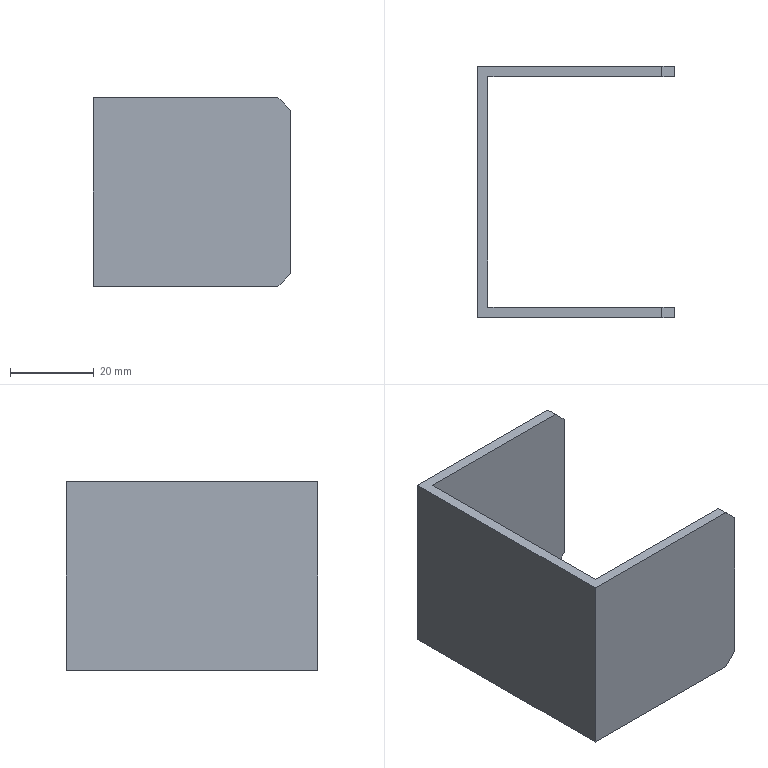Part | SolidWorks | features BaseBody 1 | 1 solid | 14 faces | box 47 x 60 x 45 mm | volume 16717 mm3 | plane 14
STEP:
#1=CARTESIAN_POINT('',(896.946,-3035.973,2067.471));
#2=VERTEX_POINT('',#1);
#3=CARTESIAN_POINT('',(896.946,-3095.973,2067.471));
#4=VERTEX_POINT('',#3);
#5=CARTESIAN_POINT('',(896.946,-3035.973,2067.471));
#6=DIRECTION('',(0.,-1.,0.));
#7=VECTOR('',#6,1000.);
#8=LINE('',#5,#7);
#9=EDGE_CURVE('',#2,#4,#8,.T.);
#10=ORIENTED_EDGE('',*,*,#9,.T.);
#11=CARTESIAN_POINT('',(896.946,-3095.973,2112.471));
#12=VERTEX_POINT('',#11);
#13=CARTESIAN_POINT('',(896.946,-3095.973,2067.471));
#14=DIRECTION('',(0.,0.,1.));
#15=VECTOR('',#14,1000.);
#16=LINE('',#13,#15);
#17=EDGE_CURVE('',#4,#12,#16,.T.);
#18=ORIENTED_EDGE('',*,*,#17,.T.);
#19=CARTESIAN_POINT('',(896.946,-3035.973,2112.471));
#20=VERTEX_POINT('',#19);
#21=CARTESIAN_POINT('',(896.946,-3035.973,2112.471));
#22=DIRECTION('',(0.,1.,0.));
#23=VECTOR('',#22,1000.);
#24=LINE('',#21,#23);
#25=EDGE_CURVE('',#12,#20,#24,.T.);
#26=ORIENTED_EDGE('',*,*,#25,.T.);
#27=CARTESIAN_POINT('',(896.946,-3035.973,2067.471));
#28=DIRECTION('',(0.,0.,-1.));
#29=VECTOR('',#28,1000.);
#30=LINE('',#27,#29);
#31=EDGE_CURVE('',#20,#2,#30,.T.);
#32=ORIENTED_EDGE('',*,*,#31,.T.);
#33=EDGE_LOOP('',(#10,#18,#26,#32));
#34=FACE_OUTER_BOUND('',#33,.T.);
#35=CARTESIAN_POINT('',(896.946,-3035.973,2067.471));
#36=DIRECTION('',(-1.,0.,0.));
#37=DIRECTION('',(0.,0.,1.));
#38=AXIS2_PLACEMENT_3D('',#35,#36,#37);
#39=PLANE('',#38);
#40=ADVANCED_FACE('',(#34),#39,.T.);
#41=CARTESIAN_POINT('',(940.946,-3095.973,2067.471));
#42=VERTEX_POINT('',#41);
#43=CARTESIAN_POINT('',(943.946,-3095.973,2070.471));
#44=VERTEX_POINT('',#43);
#45=CARTESIAN_POINT('',(940.946,-3095.973,2067.471));
#46=DIRECTION('',(0.7071,0.,0.7071));
#47=VECTOR('',#46,1000.);
#48=LINE('',#45,#47);
#49=EDGE_CURVE('',#42,#44,#48,.T.);
#50=ORIENTED_EDGE('',*,*,#49,.T.);
#51=CARTESIAN_POINT('',(943.946,-3095.973,2109.471));
#52=VERTEX_POINT('',#51);
#53=CARTESIAN_POINT('',(943.946,-3095.973,2067.471));
#54=DIRECTION('',(0.,0.,1.));
#55=VECTOR('',#54,1000.);
#56=LINE('',#53,#55);
#57=EDGE_CURVE('',#44,#52,#56,.T.);
#58=ORIENTED_EDGE('',*,*,#57,.T.);
#59=CARTESIAN_POINT('',(940.946,-3095.973,2112.471));
#60=VERTEX_POINT('',#59);
#61=CARTESIAN_POINT('',(943.946,-3095.973,2109.471));
#62=DIRECTION('',(-0.7071,0.,0.7071));
#63=VECTOR('',#62,1000.);
#64=LINE('',#61,#63);
#65=EDGE_CURVE('',#52,#60,#64,.T.);
#66=ORIENTED_EDGE('',*,*,#65,.T.);
#67=CARTESIAN_POINT('',(896.946,-3095.973,2112.471));
#68=DIRECTION('',(-1.,0.,0.));
#69=VECTOR('',#68,1000.);
#70=LINE('',#67,#69);
#71=EDGE_CURVE('',#60,#12,#70,.T.);
#72=ORIENTED_EDGE('',*,*,#71,.T.);
#73=ORIENTED_EDGE('',*,*,#17,.F.);
#74=CARTESIAN_POINT('',(896.946,-3095.973,2067.471));
#75=DIRECTION('',(1.,0.,0.));
#76=VECTOR('',#75,1000.);
#77=LINE('',#74,#76);
#78=EDGE_CURVE('',#4,#42,#77,.T.);
#79=ORIENTED_EDGE('',*,*,#78,.T.);
#80=EDGE_LOOP('',(#50,#58,#66,#72,#73,#79));
#81=FACE_OUTER_BOUND('',#80,.T.);
#82=CARTESIAN_POINT('',(896.946,-3095.973,2067.471));
#83=DIRECTION('',(0.,-1.,0.));
#84=DIRECTION('',(0.,0.,-1.));
#85=AXIS2_PLACEMENT_3D('',#82,#83,#84);
#86=PLANE('',#85);
#87=ADVANCED_FACE('',(#81),#86,.T.);
#88=CARTESIAN_POINT('',(899.446,-3038.473,2067.471));
#89=VERTEX_POINT('',#88);
#90=CARTESIAN_POINT('',(940.946,-3038.473,2067.471));
#91=VERTEX_POINT('',#90);
#92=CARTESIAN_POINT('',(912.735,-3038.473,2067.471));
#93=DIRECTION('',(1.,0.,0.));
#94=VECTOR('',#93,1000.);
#95=LINE('',#92,#94);
#96=EDGE_CURVE('',#89,#91,#95,.T.);
#97=ORIENTED_EDGE('',*,*,#96,.F.);
#98=CARTESIAN_POINT('',(899.446,-3093.473,2067.471));
#99=VERTEX_POINT('',#98);
#100=CARTESIAN_POINT('',(899.446,-3065.973,2067.471));
#101=DIRECTION('',(0.,1.,0.));
#102=VECTOR('',#101,1000.);
#103=LINE('',#100,#102);
#104=EDGE_CURVE('',#99,#89,#103,.T.);
#105=ORIENTED_EDGE('',*,*,#104,.F.);
#106=CARTESIAN_POINT('',(940.946,-3093.473,2067.471));
#107=VERTEX_POINT('',#106);
#108=CARTESIAN_POINT('',(912.735,-3093.473,2067.471));
#109=DIRECTION('',(-1.,0.,0.));
#110=VECTOR('',#109,1000.);
#111=LINE('',#108,#110);
#112=EDGE_CURVE('',#107,#99,#111,.T.);
#113=ORIENTED_EDGE('',*,*,#112,.F.);
#114=CARTESIAN_POINT('',(940.946,-3065.973,2067.471));
#115=DIRECTION('',(0.,1.,0.));
#116=VECTOR('',#115,1000.);
#117=LINE('',#114,#116);
#118=EDGE_CURVE('',#42,#107,#117,.T.);
#119=ORIENTED_EDGE('',*,*,#118,.F.);
#120=ORIENTED_EDGE('',*,*,#78,.F.);
#121=ORIENTED_EDGE('',*,*,#9,.F.);
#122=CARTESIAN_POINT('',(940.946,-3035.973,2067.471));
#123=VERTEX_POINT('',#122);
#124=CARTESIAN_POINT('',(912.735,-3035.973,2067.471));
#125=DIRECTION('',(-1.,0.,0.));
#126=VECTOR('',#125,1000.);
#127=LINE('',#124,#126);
#128=EDGE_CURVE('',#123,#2,#127,.T.);
#129=ORIENTED_EDGE('',*,*,#128,.F.);
#130=CARTESIAN_POINT('',(940.946,-3065.973,2067.471));
#131=DIRECTION('',(0.,1.,0.));
#132=VECTOR('',#131,1000.);
#133=LINE('',#130,#132);
#134=EDGE_CURVE('',#91,#123,#133,.T.);
#135=ORIENTED_EDGE('',*,*,#134,.F.);
#136=EDGE_LOOP('',(#97,#105,#113,#119,#120,#121,#129,#135));
#137=FACE_OUTER_BOUND('',#136,.T.);
#138=CARTESIAN_POINT('',(912.735,-3065.973,2067.471));
#139=DIRECTION('',(0.,0.,1.));
#140=DIRECTION('',(1.,0.,0.));
#141=AXIS2_PLACEMENT_3D('',#138,#139,#140);
#142=PLANE('',#141);
#143=ADVANCED_FACE('',(#137),#142,.F.);
#144=ORIENTED_EDGE('',*,*,#31,.F.);
#145=CARTESIAN_POINT('',(940.946,-3035.973,2112.471));
#146=VERTEX_POINT('',#145);
#147=CARTESIAN_POINT('',(943.946,-3035.973,2112.471));
#148=DIRECTION('',(1.,0.,0.));
#149=VECTOR('',#148,1000.);
#150=LINE('',#147,#149);
#151=EDGE_CURVE('',#20,#146,#150,.T.);
#152=ORIENTED_EDGE('',*,*,#151,.T.);
#153=CARTESIAN_POINT('',(943.946,-3035.973,2109.471));
#154=VERTEX_POINT('',#153);
#155=CARTESIAN_POINT('',(940.946,-3035.973,2112.471));
#156=DIRECTION('',(0.7071,0.,-0.7071));
#157=VECTOR('',#156,1000.);
#158=LINE('',#155,#157);
#159=EDGE_CURVE('',#146,#154,#158,.T.);
#160=ORIENTED_EDGE('',*,*,#159,.T.);
#161=CARTESIAN_POINT('',(943.946,-3035.973,2070.471));
#162=VERTEX_POINT('',#161);
#163=CARTESIAN_POINT('',(943.946,-3035.973,2067.471));
#164=DIRECTION('',(0.,0.,-1.));
#165=VECTOR('',#164,1000.);
#166=LINE('',#163,#165);
#167=EDGE_CURVE('',#154,#162,#166,.T.);
#168=ORIENTED_EDGE('',*,*,#167,.T.);
#169=CARTESIAN_POINT('',(943.946,-3035.973,2070.471));
#170=DIRECTION('',(-0.7071,0.,-0.7071));
#171=VECTOR('',#170,1000.);
#172=LINE('',#169,#171);
#173=EDGE_CURVE('',#162,#123,#172,.T.);
#174=ORIENTED_EDGE('',*,*,#173,.T.);
#175=ORIENTED_EDGE('',*,*,#128,.T.);
#176=EDGE_LOOP('',(#144,#152,#160,#168,#174,#175));
#177=FACE_OUTER_BOUND('',#176,.T.);
#178=CARTESIAN_POINT('',(943.946,-3035.973,2067.471));
#179=DIRECTION('',(0.,1.,0.));
#180=DIRECTION('',(0.,0.,1.));
#181=AXIS2_PLACEMENT_3D('',#178,#179,#180);
#182=PLANE('',#181);
#183=ADVANCED_FACE('',(#177),#182,.T.);
#184=CARTESIAN_POINT('',(899.446,-3093.473,2112.471));
#185=VERTEX_POINT('',#184);
#186=CARTESIAN_POINT('',(899.446,-3038.473,2112.471));
#187=VERTEX_POINT('',#186);
#188=CARTESIAN_POINT('',(899.446,-3065.973,2112.471));
#189=DIRECTION('',(0.,1.,0.));
#190=VECTOR('',#189,1000.);
#191=LINE('',#188,#190);
#192=EDGE_CURVE('',#185,#187,#191,.T.);
#193=ORIENTED_EDGE('',*,*,#192,.T.);
#194=CARTESIAN_POINT('',(940.946,-3038.473,2112.471));
#195=VERTEX_POINT('',#194);
#196=CARTESIAN_POINT('',(912.735,-3038.473,2112.471));
#197=DIRECTION('',(1.,0.,0.));
#198=VECTOR('',#197,1000.);
#199=LINE('',#196,#198);
#200=EDGE_CURVE('',#187,#195,#199,.T.);
#201=ORIENTED_EDGE('',*,*,#200,.T.);
#202=CARTESIAN_POINT('',(940.946,-3065.973,2112.471));
#203=DIRECTION('',(0.,1.,0.));
#204=VECTOR('',#203,1000.);
#205=LINE('',#202,#204);
#206=EDGE_CURVE('',#195,#146,#205,.T.);
#207=ORIENTED_EDGE('',*,*,#206,.T.);
#208=ORIENTED_EDGE('',*,*,#151,.F.);
#209=ORIENTED_EDGE('',*,*,#25,.F.);
#210=ORIENTED_EDGE('',*,*,#71,.F.);
#211=CARTESIAN_POINT('',(940.946,-3093.473,2112.471));
#212=VERTEX_POINT('',#211);
#213=CARTESIAN_POINT('',(940.946,-3065.973,2112.471));
#214=DIRECTION('',(0.,1.,0.));
#215=VECTOR('',#214,1000.);
#216=LINE('',#213,#215);
#217=EDGE_CURVE('',#60,#212,#216,.T.);
#218=ORIENTED_EDGE('',*,*,#217,.T.);
#219=CARTESIAN_POINT('',(912.735,-3093.473,2112.471));
#220=DIRECTION('',(-1.,0.,0.));
#221=VECTOR('',#220,1000.);
#222=LINE('',#219,#221);
#223=EDGE_CURVE('',#212,#185,#222,.T.);
#224=ORIENTED_EDGE('',*,*,#223,.T.);
#225=EDGE_LOOP('',(#193,#201,#207,#208,#209,#210,#218,#224));
#226=FACE_OUTER_BOUND('',#225,.T.);
#227=CARTESIAN_POINT('',(912.735,-3065.973,2112.471));
#228=DIRECTION('',(0.,0.,1.));
#229=DIRECTION('',(1.,0.,0.));
#230=AXIS2_PLACEMENT_3D('',#227,#228,#229);
#231=PLANE('',#230);
#232=ADVANCED_FACE('',(#226),#231,.T.);
#233=CARTESIAN_POINT('',(943.946,-3093.473,2070.471));
#234=VERTEX_POINT('',#233);
#235=CARTESIAN_POINT('',(943.946,-3095.973,2070.471));
#236=DIRECTION('',(0.,1.,0.));
#237=VECTOR('',#236,1000.);
#238=LINE('',#235,#237);
#239=EDGE_CURVE('',#44,#234,#238,.T.);
#240=ORIENTED_EDGE('',*,*,#239,.T.);
#241=CARTESIAN_POINT('',(943.946,-3093.473,2109.471));
#242=VERTEX_POINT('',#241);
#243=CARTESIAN_POINT('',(943.946,-3093.473,2067.471));
#244=DIRECTION('',(0.,0.,1.));
#245=VECTOR('',#244,1000.);
#246=LINE('',#243,#245);
#247=EDGE_CURVE('',#234,#242,#246,.T.);
#248=ORIENTED_EDGE('',*,*,#247,.T.);
#249=CARTESIAN_POINT('',(943.946,-3095.973,2109.471));
#250=DIRECTION('',(0.,-1.,0.));
#251=VECTOR('',#250,1000.);
#252=LINE('',#249,#251);
#253=EDGE_CURVE('',#242,#52,#252,.T.);
#254=ORIENTED_EDGE('',*,*,#253,.T.);
#255=ORIENTED_EDGE('',*,*,#57,.F.);
#256=EDGE_LOOP('',(#240,#248,#254,#255));
#257=FACE_OUTER_BOUND('',#256,.T.);
#258=CARTESIAN_POINT('',(943.946,-3095.973,2067.471));
#259=DIRECTION('',(1.,0.,0.));
#260=DIRECTION('',(0.,0.,-1.));
#261=AXIS2_PLACEMENT_3D('',#258,#259,#260);
#262=PLANE('',#261);
#263=ADVANCED_FACE('',(#257),#262,.T.);
#264=ORIENTED_EDGE('',*,*,#118,.T.);
#265=CARTESIAN_POINT('',(943.946,-3093.473,2070.471));
#266=DIRECTION('',(-0.7071,0.,-0.7071));
#267=VECTOR('',#266,1000.);
#268=LINE('',#265,#267);
#269=EDGE_CURVE('',#234,#107,#268,.T.);
#270=ORIENTED_EDGE('',*,*,#269,.F.);
#271=ORIENTED_EDGE('',*,*,#239,.F.);
#272=ORIENTED_EDGE('',*,*,#49,.F.);
#273=EDGE_LOOP('',(#264,#270,#271,#272));
#274=FACE_OUTER_BOUND('',#273,.T.);
#275=CARTESIAN_POINT('',(943.946,-2900.175,2070.471));
#276=DIRECTION('',(-0.7071,0.,0.7071));
#277=DIRECTION('',(0.7071,0.,0.7071));
#278=AXIS2_PLACEMENT_3D('',#275,#276,#277);
#279=PLANE('',#278);
#280=ADVANCED_FACE('',(#274),#279,.F.);
#281=ORIENTED_EDGE('',*,*,#253,.F.);
#282=CARTESIAN_POINT('',(943.946,-3093.473,2109.471));
#283=DIRECTION('',(0.7071,0.,-0.7071));
#284=VECTOR('',#283,1000.);
#285=LINE('',#282,#284);
#286=EDGE_CURVE('',#212,#242,#285,.T.);
#287=ORIENTED_EDGE('',*,*,#286,.F.);
#288=ORIENTED_EDGE('',*,*,#217,.F.);
#289=ORIENTED_EDGE('',*,*,#65,.F.);
#290=EDGE_LOOP('',(#281,#287,#288,#289));
#291=FACE_OUTER_BOUND('',#290,.T.);
#292=CARTESIAN_POINT('',(943.946,-2900.175,2109.471));
#293=DIRECTION('',(-0.7071,0.,-0.7071));
#294=DIRECTION('',(-0.7071,0.,0.7071));
#295=AXIS2_PLACEMENT_3D('',#292,#293,#294);
#296=PLANE('',#295);
#297=ADVANCED_FACE('',(#291),#296,.F.);
#298=CARTESIAN_POINT('',(943.946,-3038.473,2070.471));
#299=VERTEX_POINT('',#298);
#300=CARTESIAN_POINT('',(943.946,-2900.175,2070.471));
#301=DIRECTION('',(0.,1.,0.));
#302=VECTOR('',#301,1000.);
#303=LINE('',#300,#302);
#304=EDGE_CURVE('',#299,#162,#303,.T.);
#305=ORIENTED_EDGE('',*,*,#304,.F.);
#306=CARTESIAN_POINT('',(943.946,-3038.473,2070.471));
#307=DIRECTION('',(0.7071,0.,0.7071));
#308=VECTOR('',#307,1000.);
#309=LINE('',#306,#308);
#310=EDGE_CURVE('',#91,#299,#309,.T.);
#311=ORIENTED_EDGE('',*,*,#310,.F.);
#312=ORIENTED_EDGE('',*,*,#134,.T.);
#313=ORIENTED_EDGE('',*,*,#173,.F.);
#314=EDGE_LOOP('',(#305,#311,#312,#313));
#315=FACE_OUTER_BOUND('',#314,.T.);
#316=CARTESIAN_POINT('',(943.946,-2900.175,2070.471));
#317=DIRECTION('',(-0.7071,0.,0.7071));
#318=DIRECTION('',(0.7071,0.,0.7071));
#319=AXIS2_PLACEMENT_3D('',#316,#317,#318);
#320=PLANE('',#319);
#321=ADVANCED_FACE('',(#315),#320,.F.);
#322=ORIENTED_EDGE('',*,*,#310,.T.);
#323=CARTESIAN_POINT('',(943.946,-3038.473,2109.471));
#324=VERTEX_POINT('',#323);
#325=CARTESIAN_POINT('',(943.946,-3038.473,2067.471));
#326=DIRECTION('',(0.,0.,1.));
#327=VECTOR('',#326,1000.);
#328=LINE('',#325,#327);
#329=EDGE_CURVE('',#299,#324,#328,.T.);
#330=ORIENTED_EDGE('',*,*,#329,.T.);
#331=CARTESIAN_POINT('',(943.946,-3038.473,2109.471));
#332=DIRECTION('',(-0.7071,0.,0.7071));
#333=VECTOR('',#332,1000.);
#334=LINE('',#331,#333);
#335=EDGE_CURVE('',#324,#195,#334,.T.);
#336=ORIENTED_EDGE('',*,*,#335,.T.);
#337=ORIENTED_EDGE('',*,*,#200,.F.);
#338=CARTESIAN_POINT('',(899.446,-3038.473,2067.471));
#339=DIRECTION('',(0.,0.,-1.));
#340=VECTOR('',#339,1000.);
#341=LINE('',#338,#340);
#342=EDGE_CURVE('',#187,#89,#341,.T.);
#343=ORIENTED_EDGE('',*,*,#342,.T.);
#344=ORIENTED_EDGE('',*,*,#96,.T.);
#345=EDGE_LOOP('',(#322,#330,#336,#337,#343,#344));
#346=FACE_OUTER_BOUND('',#345,.T.);
#347=CARTESIAN_POINT('',(899.446,-3038.473,2067.471));
#348=DIRECTION('',(0.,-1.,0.));
#349=DIRECTION('',(0.,0.,-1.));
#350=AXIS2_PLACEMENT_3D('',#347,#348,#349);
#351=PLANE('',#350);
#352=ADVANCED_FACE('',(#346),#351,.T.);
#353=ORIENTED_EDGE('',*,*,#104,.T.);
#354=ORIENTED_EDGE('',*,*,#342,.F.);
#355=ORIENTED_EDGE('',*,*,#192,.F.);
#356=CARTESIAN_POINT('',(899.446,-3093.473,2067.471));
#357=DIRECTION('',(0.,0.,-1.));
#358=VECTOR('',#357,1000.);
#359=LINE('',#356,#358);
#360=EDGE_CURVE('',#185,#99,#359,.T.);
#361=ORIENTED_EDGE('',*,*,#360,.T.);
#362=EDGE_LOOP('',(#353,#354,#355,#361));
#363=FACE_OUTER_BOUND('',#362,.T.);
#364=CARTESIAN_POINT('',(899.446,-3093.473,2067.471));
#365=DIRECTION('',(1.,0.,0.));
#366=DIRECTION('',(0.,0.,-1.));
#367=AXIS2_PLACEMENT_3D('',#364,#365,#366);
#368=PLANE('',#367);
#369=ADVANCED_FACE('',(#363),#368,.T.);
#370=ORIENTED_EDGE('',*,*,#360,.F.);
#371=ORIENTED_EDGE('',*,*,#223,.F.);
#372=ORIENTED_EDGE('',*,*,#286,.T.);
#373=ORIENTED_EDGE('',*,*,#247,.F.);
#374=ORIENTED_EDGE('',*,*,#269,.T.);
#375=ORIENTED_EDGE('',*,*,#112,.T.);
#376=EDGE_LOOP('',(#370,#371,#372,#373,#374,#375));
#377=FACE_OUTER_BOUND('',#376,.T.);
#378=CARTESIAN_POINT('',(943.946,-3093.473,2067.471));
#379=DIRECTION('',(0.,1.,0.));
#380=DIRECTION('',(0.,0.,1.));
#381=AXIS2_PLACEMENT_3D('',#378,#379,#380);
#382=PLANE('',#381);
#383=ADVANCED_FACE('',(#377),#382,.T.);
#384=ORIENTED_EDGE('',*,*,#304,.T.);
#385=ORIENTED_EDGE('',*,*,#167,.F.);
#386=CARTESIAN_POINT('',(943.946,-3038.473,2109.471));
#387=DIRECTION('',(0.,-1.,0.));
#388=VECTOR('',#387,1000.);
#389=LINE('',#386,#388);
#390=EDGE_CURVE('',#154,#324,#389,.T.);
#391=ORIENTED_EDGE('',*,*,#390,.T.);
#392=ORIENTED_EDGE('',*,*,#329,.F.);
#393=EDGE_LOOP('',(#384,#385,#391,#392));
#394=FACE_OUTER_BOUND('',#393,.T.);
#395=CARTESIAN_POINT('',(943.946,-3038.473,2067.471));
#396=DIRECTION('',(1.,0.,0.));
#397=DIRECTION('',(0.,0.,-1.));
#398=AXIS2_PLACEMENT_3D('',#395,#396,#397);
#399=PLANE('',#398);
#400=ADVANCED_FACE('',(#394),#399,.T.);
#401=ORIENTED_EDGE('',*,*,#206,.F.);
#402=ORIENTED_EDGE('',*,*,#335,.F.);
#403=ORIENTED_EDGE('',*,*,#390,.F.);
#404=ORIENTED_EDGE('',*,*,#159,.F.);
#405=EDGE_LOOP('',(#401,#402,#403,#404));
#406=FACE_OUTER_BOUND('',#405,.T.);
#407=CARTESIAN_POINT('',(943.946,-2900.175,2109.471));
#408=DIRECTION('',(-0.7071,0.,-0.7071));
#409=DIRECTION('',(-0.7071,0.,0.7071));
#410=AXIS2_PLACEMENT_3D('',#407,#408,#409);
#411=PLANE('',#410);
#412=ADVANCED_FACE('',(#406),#411,.F.);
#413=CLOSED_SHELL('',(#40,#87,#143,#183,#232,#263,#280,#297,#321,#352,#369,#383,#400,#412));
#414=MANIFOLD_SOLID_BREP('',#413);
#415=CARTESIAN_POINT('',(0.,0.,0.));
#416=DIRECTION('',(0.,0.,1.));
#417=DIRECTION('',(1.,0.,0.));
#418=AXIS2_PLACEMENT_3D('',#415,#416,#417);
#419=(LENGTH_UNIT()NAMED_UNIT(*)SI_UNIT(.MILLI.,.METRE.));
#420=UNCERTAINTY_MEASURE_WITH_UNIT(LENGTH_MEASURE(0.00001),#419,'','');
#421=(NAMED_UNIT(*)PLANE_ANGLE_UNIT()SI_UNIT($,.RADIAN.));
#422=(NAMED_UNIT(*)SI_UNIT($,.STERADIAN.)SOLID_ANGLE_UNIT());
#423=(GEOMETRIC_REPRESENTATION_CONTEXT(3)GLOBAL_UNCERTAINTY_ASSIGNED_CONTEXT((#420))GLOBAL_UNIT_ASSIGNED_CONTEXT((#419,#421,#422))REPRESENTATION_CONTEXT('',''));
#424=ADVANCED_BREP_SHAPE_REPRESENTATION('',(#414,#418),#423);